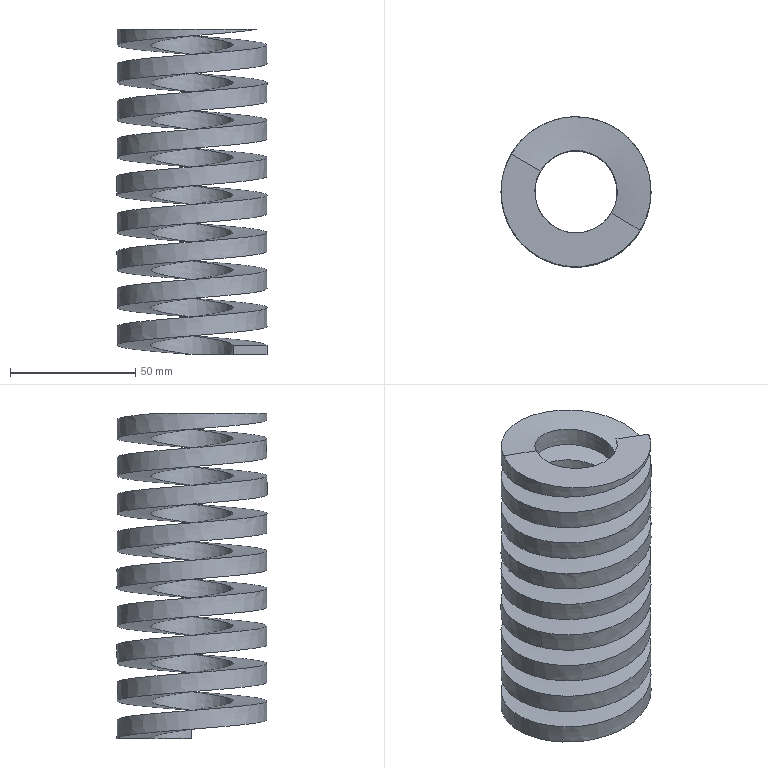Part | STEP file | FTH60.00-145.00 | 1 solid | 7 faces | box 60 x 60.001 x 130 mm | volume 125930 mm3 | spline 5 | plane 2